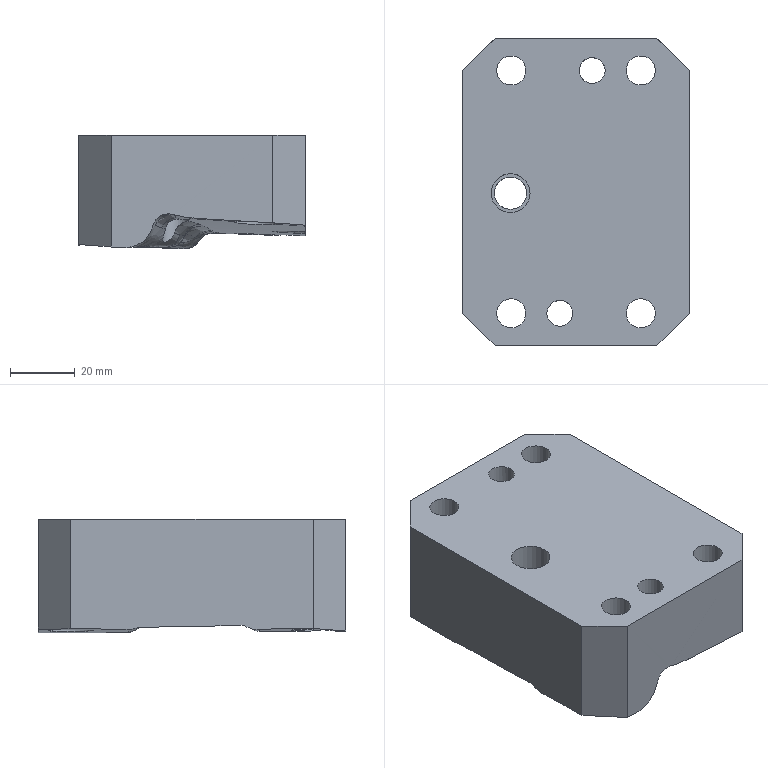Part | NX | features solid 2 | 1 solid | 80 faces | box 70 x 95.008 x 35.13 mm | volume 178442 mm3 | spline 54 | plane 14 | cylinder 12 | commonest cylinder face diameters 9 x4 14 x4 8 x2 10 x1 12 x1